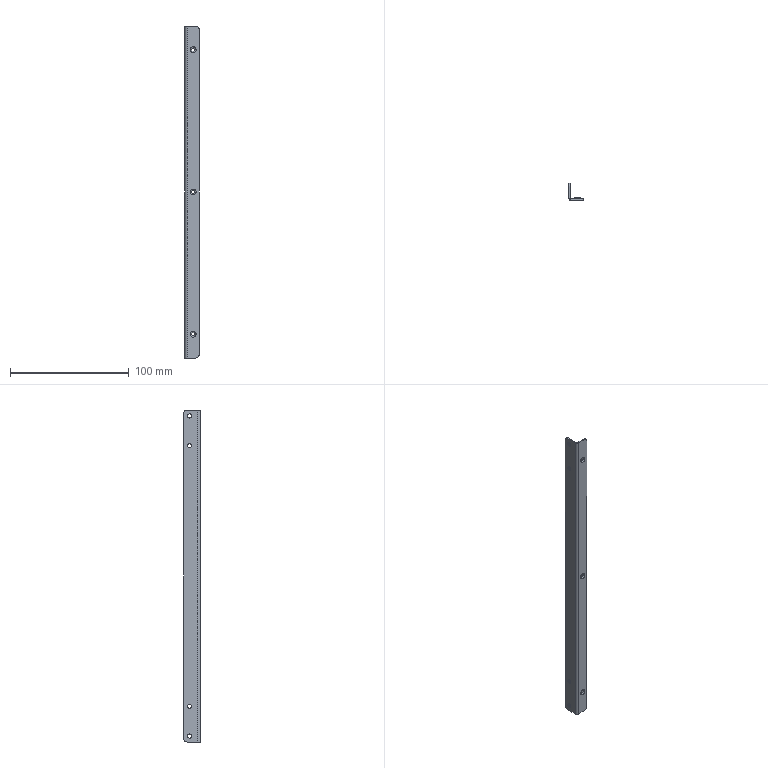Part | SolidWorks | features BaseBody 1 | 1 solid | 43 faces | box 12 x 14.1 x 280 mm | volume 6830 mm3 | cylinder 26 | plane 11 | spline 6 | commonest cylinder face diameters 3.5 x8 3 x6 5 x6 6 x4 2 x1 4 x1